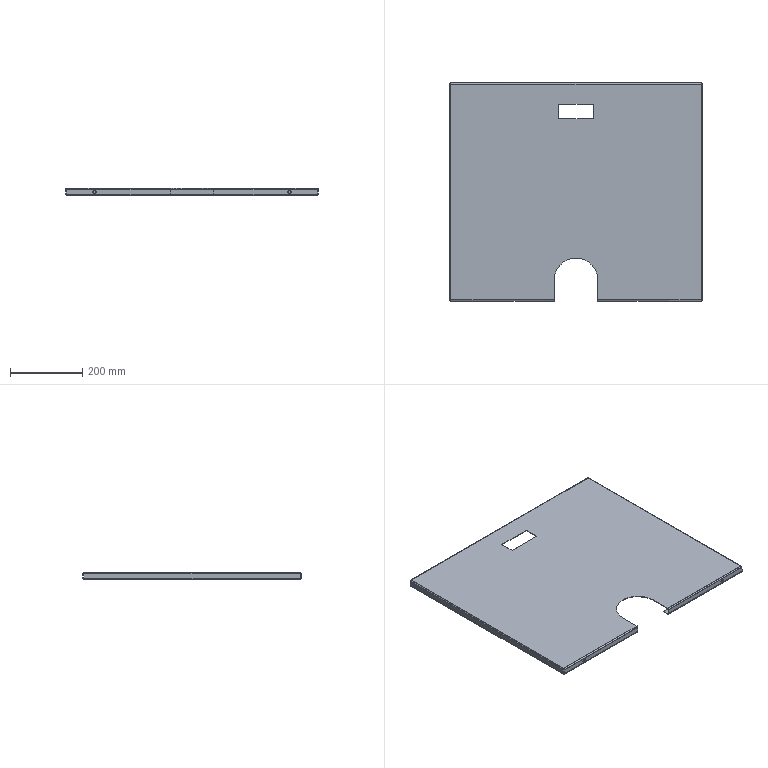Part | SolidWorks | features EdgeFlange 2, FlatPattern 1, HoleWzd 1, ICE 1, SMBaseFlange 1, SheetMetal 1 | 1 solid | 98 faces | box 700 x 605 x 20 mm | volume 736343 mm3 | plane 57 | cylinder 25 | spline 16 | commonest cylinder face diameters 4 x10 7 x10 9 x4 120 x1